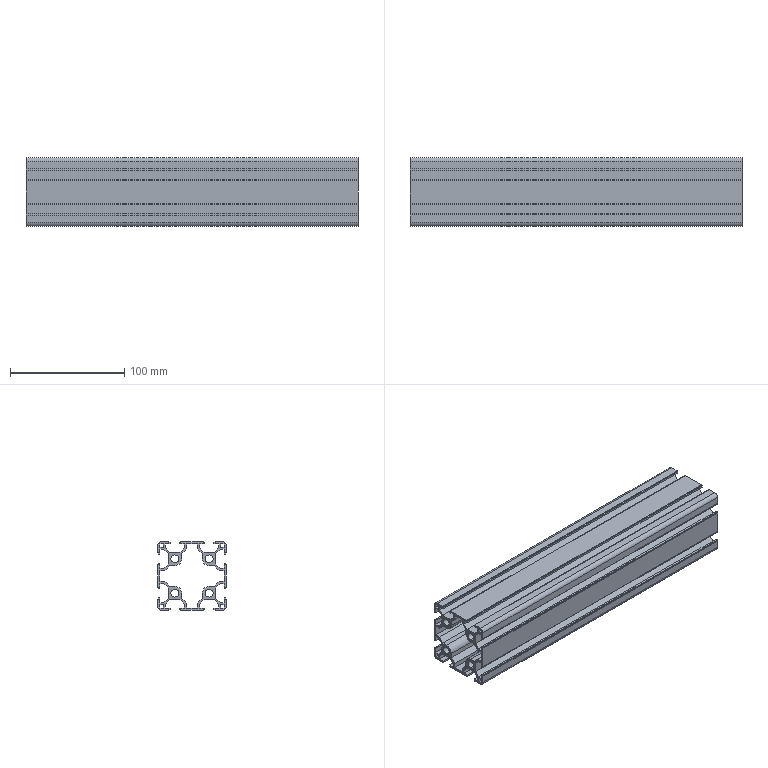Part | STEP file | Square aluminium tube PN_0026_Default <Machined> | 1 solid | 178 faces | box 290 x 60 x 60 mm | volume 266913 mm3 | plane 162 | cylinder 16 | commonest cylinder face diameters 6.8 x8 6.76 x4 11.828 x4